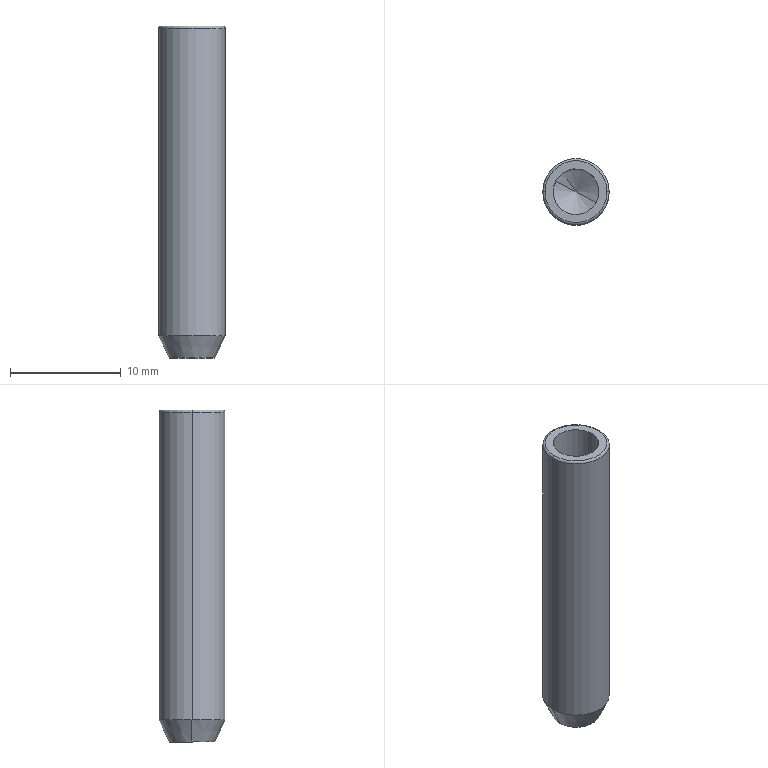Part | CATIA | 1 solid | 12 faces | box 6 x 6 x 30 mm | volume 692.749 mm3 | cone 4 | cylinder 4 | plane 2 | torus 2 | commonest cylinder face diameters 4.134 x2 6 x2
STEP:
#1=CARTESIAN_POINT('',(0.,0.,18.807));
#2=VERTEX_POINT('',#1);
#3=CARTESIAN_POINT('',(-1.814,0.991,20.));
#4=VERTEX_POINT('',#3);
#5=CARTESIAN_POINT('',(-0.907,0.4955,19.403));
#6=DIRECTION('',(-0.76,0.4152,0.5));
#7=VECTOR('',#6,1.);
#8=LINE('',#5,#7);
#9=EDGE_CURVE('',#2,#4,#8,.T.);
#10=ORIENTED_EDGE('',*,*,#9,.T.);
#11=CARTESIAN_POINT('',(1.814,-0.991,20.));
#12=VERTEX_POINT('',#11);
#13=CARTESIAN_POINT('',(0.,0.,20.));
#14=DIRECTION('',(0.,0.,1.));
#15=AXIS2_PLACEMENT_3D('',#13,#14,$);
#16=CIRCLE('',#15,2.067);
#17=EDGE_CURVE('',#12,#4,#16,.F.);
#18=ORIENTED_EDGE('',*,*,#17,.F.);
#19=CARTESIAN_POINT('',(0.907,-0.4955,19.403));
#20=DIRECTION('',(0.76,-0.4152,0.5));
#21=VECTOR('',#20,1.);
#22=LINE('',#19,#21);
#23=EDGE_CURVE('',#2,#12,#22,.T.);
#24=ORIENTED_EDGE('',*,*,#23,.F.);
#25=EDGE_LOOP('',(#10,#18,#24));
#26=FACE_OUTER_BOUND('',#25,.T.);
#27=CARTESIAN_POINT('',(0.,0.,18.807));
#28=DIRECTION('',(0.,0.,1.));
#29=DIRECTION('',(0.8776,-0.4794,0.));
#30=AXIS2_PLACEMENT_3D('',#27,#28,#29);
#31=CONICAL_SURFACE('',#30,0.,1.047);
#32=ADVANCED_FACE('',(#26),#31,.F.);
#33=CARTESIAN_POINT('',(-2.8,0.000000213,30.));
#34=VERTEX_POINT('',#33);
#35=CARTESIAN_POINT('',(2.8,0.,30.));
#36=VERTEX_POINT('',#35);
#37=CARTESIAN_POINT('',(0.,0.,30.));
#38=DIRECTION('',(0.,0.,1.));
#39=AXIS2_PLACEMENT_3D('',#37,#38,$);
#40=CIRCLE('',#39,2.8);
#41=EDGE_CURVE('',#34,#36,#40,.T.);
#42=ORIENTED_EDGE('',*,*,#41,.T.);
#43=CARTESIAN_POINT('',(0.,0.,30.));
#44=DIRECTION('',(0.,0.,1.));
#45=AXIS2_PLACEMENT_3D('',#43,#44,$);
#46=CIRCLE('',#45,2.8);
#47=EDGE_CURVE('',#36,#34,#46,.T.);
#48=ORIENTED_EDGE('',*,*,#47,.T.);
#49=EDGE_LOOP('',(#42,#48));
#50=FACE_OUTER_BOUND('',#49,.T.);
#51=CARTESIAN_POINT('',(-1.814,0.991,30.));
#52=VERTEX_POINT('',#51);
#53=CARTESIAN_POINT('',(1.814,-0.991,30.));
#54=VERTEX_POINT('',#53);
#55=CARTESIAN_POINT('',(0.,0.,30.));
#56=DIRECTION('',(0.,0.,1.));
#57=AXIS2_PLACEMENT_3D('',#55,#56,$);
#58=CIRCLE('',#57,2.067);
#59=EDGE_CURVE('',#52,#54,#58,.T.);
#60=ORIENTED_EDGE('',*,*,#59,.F.);
#61=CARTESIAN_POINT('',(0.,0.,30.));
#62=DIRECTION('',(0.,0.,1.));
#63=AXIS2_PLACEMENT_3D('',#61,#62,$);
#64=CIRCLE('',#63,2.067);
#65=EDGE_CURVE('',#54,#52,#64,.T.);
#66=ORIENTED_EDGE('',*,*,#65,.F.);
#67=EDGE_LOOP('',(#60,#66));
#68=FACE_BOUND('',#67,.T.);
#69=CARTESIAN_POINT('',(0.,0.,30.));
#70=DIRECTION('',(0.,0.,1.));
#71=DIRECTION('',(1.,0.,0.));
#72=AXIS2_PLACEMENT_3D('',#69,#70,#71);
#73=PLANE('',#72);
#74=ADVANCED_FACE('',(#50,#68),#73,.T.);
#75=CARTESIAN_POINT('',(-3.,0.,29.8));
#76=VERTEX_POINT('',#75);
#77=CARTESIAN_POINT('',(-2.8,0.,29.8));
#78=DIRECTION('',(0.,1.,0.));
#79=AXIS2_PLACEMENT_3D('',#77,#78,$);
#80=CIRCLE('',#79,0.2);
#81=EDGE_CURVE('',#34,#76,#80,.F.);
#82=ORIENTED_EDGE('',*,*,#81,.T.);
#83=CARTESIAN_POINT('',(3.,0.,29.8));
#84=VERTEX_POINT('',#83);
#85=CARTESIAN_POINT('',(0.,0.,29.8));
#86=DIRECTION('',(0.,0.,1.));
#87=AXIS2_PLACEMENT_3D('',#85,#86,$);
#88=CIRCLE('',#87,3.);
#89=EDGE_CURVE('',#76,#84,#88,.T.);
#90=ORIENTED_EDGE('',*,*,#89,.T.);
#91=CARTESIAN_POINT('',(2.8,0.,29.8));
#92=DIRECTION('',(0.,-1.,0.));
#93=AXIS2_PLACEMENT_3D('',#91,#92,$);
#94=CIRCLE('',#93,0.2);
#95=EDGE_CURVE('',#36,#84,#94,.F.);
#96=ORIENTED_EDGE('',*,*,#95,.F.);
#97=ORIENTED_EDGE('',*,*,#41,.F.);
#98=EDGE_LOOP('',(#82,#90,#96,#97));
#99=FACE_OUTER_BOUND('',#98,.T.);
#100=CARTESIAN_POINT('',(0.,0.,29.8));
#101=DIRECTION('',(0.,0.,1.));
#102=DIRECTION('',(-0.9941,0.1086,0.));
#103=AXIS2_PLACEMENT_3D('',#100,#101,#102);
#104=TOROIDAL_SURFACE('',#103,2.8,0.2);
#105=ADVANCED_FACE('',(#99),#104,.T.);
#106=ORIENTED_EDGE('',*,*,#95,.T.);
#107=CARTESIAN_POINT('',(0.,0.,29.8));
#108=DIRECTION('',(0.,0.,1.));
#109=AXIS2_PLACEMENT_3D('',#107,#108,$);
#110=CIRCLE('',#109,3.);
#111=EDGE_CURVE('',#84,#76,#110,.T.);
#112=ORIENTED_EDGE('',*,*,#111,.T.);
#113=ORIENTED_EDGE('',*,*,#81,.F.);
#114=ORIENTED_EDGE('',*,*,#47,.F.);
#115=EDGE_LOOP('',(#106,#112,#113,#114));
#116=FACE_OUTER_BOUND('',#115,.T.);
#117=CARTESIAN_POINT('',(0.,0.,29.8));
#118=DIRECTION('',(0.,0.,1.));
#119=DIRECTION('',(1.,0.,0.));
#120=AXIS2_PLACEMENT_3D('',#117,#118,#119);
#121=TOROIDAL_SURFACE('',#120,2.8,0.2);
#122=ADVANCED_FACE('',(#116),#121,.T.);
#123=CARTESIAN_POINT('',(3.,0.,2.));
#124=VERTEX_POINT('',#123);
#125=CARTESIAN_POINT('',(3.,0.,15.));
#126=DIRECTION('',(0.,0.,1.));
#127=VECTOR('',#126,1.);
#128=LINE('',#125,#127);
#129=EDGE_CURVE('',#124,#84,#128,.T.);
#130=ORIENTED_EDGE('',*,*,#129,.T.);
#131=ORIENTED_EDGE('',*,*,#89,.F.);
#132=CARTESIAN_POINT('',(-3.,0.,2.));
#133=VERTEX_POINT('',#132);
#134=CARTESIAN_POINT('',(-3.,0.,15.));
#135=DIRECTION('',(0.,0.,1.));
#136=VECTOR('',#135,1.);
#137=LINE('',#134,#136);
#138=EDGE_CURVE('',#133,#76,#137,.T.);
#139=ORIENTED_EDGE('',*,*,#138,.F.);
#140=CARTESIAN_POINT('',(0.,0.,2.));
#141=DIRECTION('',(0.,0.,1.));
#142=AXIS2_PLACEMENT_3D('',#140,#141,$);
#143=CIRCLE('',#142,3.);
#144=EDGE_CURVE('',#133,#124,#143,.T.);
#145=ORIENTED_EDGE('',*,*,#144,.T.);
#146=EDGE_LOOP('',(#130,#131,#139,#145));
#147=FACE_OUTER_BOUND('',#146,.T.);
#148=CARTESIAN_POINT('',(0.,0.,15.));
#149=DIRECTION('',(0.,0.,1.));
#150=DIRECTION('',(1.,0.,0.));
#151=AXIS2_PLACEMENT_3D('',#148,#149,#150);
#152=CYLINDRICAL_SURFACE('',#151,3.);
#153=ADVANCED_FACE('',(#147),#152,.T.);
#154=ORIENTED_EDGE('',*,*,#138,.T.);
#155=ORIENTED_EDGE('',*,*,#111,.F.);
#156=ORIENTED_EDGE('',*,*,#129,.F.);
#157=CARTESIAN_POINT('',(0.,0.,2.));
#158=DIRECTION('',(0.,0.,1.));
#159=AXIS2_PLACEMENT_3D('',#157,#158,$);
#160=CIRCLE('',#159,3.);
#161=EDGE_CURVE('',#124,#133,#160,.T.);
#162=ORIENTED_EDGE('',*,*,#161,.T.);
#163=EDGE_LOOP('',(#154,#155,#156,#162));
#164=FACE_OUTER_BOUND('',#163,.T.);
#165=ADVANCED_FACE('',(#164),#152,.T.);
#166=CARTESIAN_POINT('',(-2.067,0.000000105,0.));
#167=VERTEX_POINT('',#166);
#168=CARTESIAN_POINT('',(-2.534,-0.000000291,1.));
#169=DIRECTION('',(-0.4226,-0.000000049,0.9063));
#170=VECTOR('',#169,1.);
#171=LINE('',#168,#170);
#172=EDGE_CURVE('',#133,#167,#171,.F.);
#173=ORIENTED_EDGE('',*,*,#172,.T.);
#174=CARTESIAN_POINT('',(2.067,0.,0.));
#175=VERTEX_POINT('',#174);
#176=CARTESIAN_POINT('',(0.,0.,0.));
#177=DIRECTION('',(0.,0.,1.));
#178=AXIS2_PLACEMENT_3D('',#176,#177,$);
#179=CIRCLE('',#178,2.067);
#180=EDGE_CURVE('',#167,#175,#179,.T.);
#181=ORIENTED_EDGE('',*,*,#180,.T.);
#182=CARTESIAN_POINT('',(2.534,0.,1.));
#183=DIRECTION('',(0.4226,0.,0.9063));
#184=VECTOR('',#183,1.);
#185=LINE('',#182,#184);
#186=EDGE_CURVE('',#124,#175,#185,.F.);
#187=ORIENTED_EDGE('',*,*,#186,.F.);
#188=ORIENTED_EDGE('',*,*,#144,.F.);
#189=EDGE_LOOP('',(#173,#181,#187,#188));
#190=FACE_OUTER_BOUND('',#189,.T.);
#191=CARTESIAN_POINT('',(0.,0.,-4.434));
#192=DIRECTION('',(0.,0.,1.));
#193=DIRECTION('',(-0.9405,0.3399,0.));
#194=AXIS2_PLACEMENT_3D('',#191,#192,#193);
#195=CONICAL_SURFACE('',#194,0.,0.4363);
#196=ADVANCED_FACE('',(#190),#195,.T.);
#197=ORIENTED_EDGE('',*,*,#186,.T.);
#198=CARTESIAN_POINT('',(0.,0.,0.));
#199=DIRECTION('',(0.,0.,1.));
#200=AXIS2_PLACEMENT_3D('',#198,#199,$);
#201=CIRCLE('',#200,2.067);
#202=EDGE_CURVE('',#175,#167,#201,.T.);
#203=ORIENTED_EDGE('',*,*,#202,.T.);
#204=ORIENTED_EDGE('',*,*,#172,.F.);
#205=ORIENTED_EDGE('',*,*,#161,.F.);
#206=EDGE_LOOP('',(#197,#203,#204,#205));
#207=FACE_OUTER_BOUND('',#206,.T.);
#208=CARTESIAN_POINT('',(0.,0.,-4.434));
#209=DIRECTION('',(0.,0.,1.));
#210=DIRECTION('',(1.,0.,0.));
#211=AXIS2_PLACEMENT_3D('',#208,#209,#210);
#212=CONICAL_SURFACE('',#211,0.,0.4363);
#213=ADVANCED_FACE('',(#207),#212,.T.);
#214=ORIENTED_EDGE('',*,*,#202,.F.);
#215=ORIENTED_EDGE('',*,*,#180,.F.);
#216=EDGE_LOOP('',(#214,#215));
#217=FACE_OUTER_BOUND('',#216,.T.);
#218=CARTESIAN_POINT('',(0.,0.,0.));
#219=DIRECTION('',(0.,0.,1.));
#220=DIRECTION('',(1.,0.,0.));
#221=AXIS2_PLACEMENT_3D('',#218,#219,#220);
#222=PLANE('',#221);
#223=ADVANCED_FACE('',(#217),#222,.F.);
#224=ORIENTED_EDGE('',*,*,#65,.T.);
#225=CARTESIAN_POINT('',(-1.814,0.991,25.155));
#226=DIRECTION('',(0.,0.,-1.));
#227=VECTOR('',#226,1.);
#228=LINE('',#225,#227);
#229=EDGE_CURVE('',#4,#52,#228,.F.);
#230=ORIENTED_EDGE('',*,*,#229,.F.);
#231=CARTESIAN_POINT('',(0.,0.,20.));
#232=DIRECTION('',(0.,0.,-1.));
#233=AXIS2_PLACEMENT_3D('',#231,#232,$);
#234=CIRCLE('',#233,2.067);
#235=EDGE_CURVE('',#4,#12,#234,.T.);
#236=ORIENTED_EDGE('',*,*,#235,.T.);
#237=CARTESIAN_POINT('',(1.814,-0.991,25.155));
#238=DIRECTION('',(0.,0.,-1.));
#239=VECTOR('',#238,1.);
#240=LINE('',#237,#239);
#241=EDGE_CURVE('',#12,#54,#240,.F.);
#242=ORIENTED_EDGE('',*,*,#241,.T.);
#243=EDGE_LOOP('',(#224,#230,#236,#242));
#244=FACE_OUTER_BOUND('',#243,.T.);
#245=CARTESIAN_POINT('',(0.,0.,29.9));
#246=DIRECTION('',(0.,0.,-1.));
#247=DIRECTION('',(0.8776,-0.4794,0.));
#248=AXIS2_PLACEMENT_3D('',#245,#246,#247);
#249=CYLINDRICAL_SURFACE('',#248,2.067);
#250=ADVANCED_FACE('',(#244),#249,.F.);
#251=ORIENTED_EDGE('',*,*,#59,.T.);
#252=ORIENTED_EDGE('',*,*,#241,.F.);
#253=ORIENTED_EDGE('',*,*,#17,.T.);
#254=ORIENTED_EDGE('',*,*,#229,.T.);
#255=EDGE_LOOP('',(#251,#252,#253,#254));
#256=FACE_OUTER_BOUND('',#255,.T.);
#257=ADVANCED_FACE('',(#256),#249,.F.);
#258=ORIENTED_EDGE('',*,*,#23,.T.);
#259=ORIENTED_EDGE('',*,*,#235,.F.);
#260=ORIENTED_EDGE('',*,*,#9,.F.);
#261=EDGE_LOOP('',(#258,#259,#260));
#262=FACE_OUTER_BOUND('',#261,.T.);
#263=ADVANCED_FACE('',(#262),#31,.F.);
#264=CLOSED_SHELL('',(#32,#74,#105,#122,#153,#165,#196,#213,#223,#250,#257,#263));
#265=MANIFOLD_SOLID_BREP('',#264);
#266=(LENGTH_UNIT()NAMED_UNIT(*)SI_UNIT(.MILLI.,.METRE.));
#267=UNCERTAINTY_MEASURE_WITH_UNIT(LENGTH_MEASURE(0.005),#266,'','');
#268=(NAMED_UNIT(*)PLANE_ANGLE_UNIT()SI_UNIT($,.RADIAN.));
#269=(NAMED_UNIT(*)SI_UNIT($,.STERADIAN.)SOLID_ANGLE_UNIT());
#270=(GEOMETRIC_REPRESENTATION_CONTEXT(3)GLOBAL_UNCERTAINTY_ASSIGNED_CONTEXT((#267))GLOBAL_UNIT_ASSIGNED_CONTEXT((#266,#268,#269))REPRESENTATION_CONTEXT('',''));
#271=ADVANCED_BREP_SHAPE_REPRESENTATION('',(#265),#270);